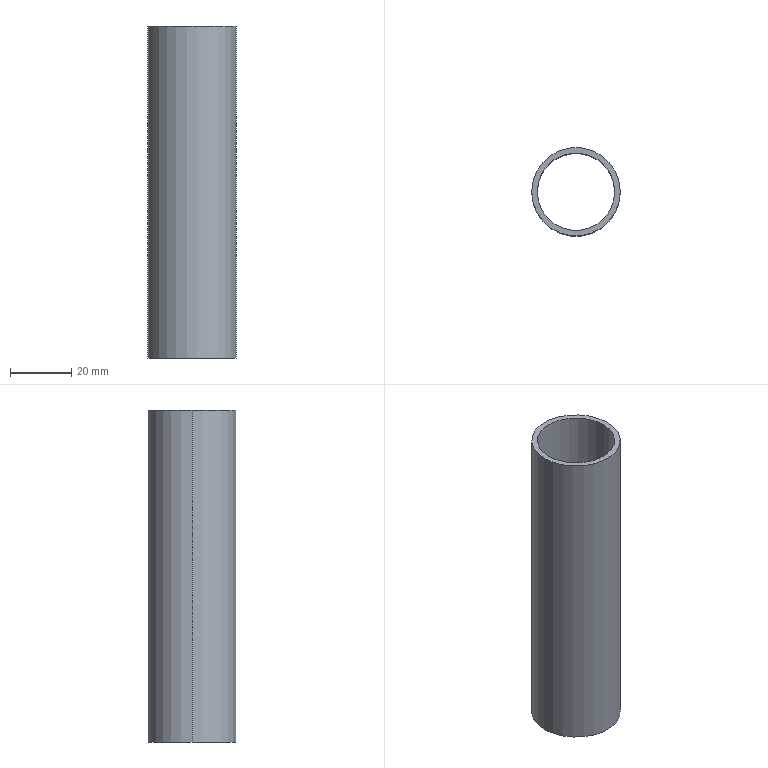Part | SolidWorks | features Extrusion 1 | 1 solid | 6 faces | box 28.8 x 28.8 x 108 mm | volume 16490 mm3 | cylinder 4 | plane 2 | commonest cylinder face diameters 25.2 x2 28.8 x2
STEP:
#1=CARTESIAN_POINT('',(-12.6,0.,108.));
#2=VERTEX_POINT('',#1);
#3=CARTESIAN_POINT('',(12.6,0.,108.));
#4=VERTEX_POINT('',#3);
#5=CARTESIAN_POINT('',(0.,0.,108.));
#6=DIRECTION('',(0.,0.,1.));
#7=DIRECTION('',(1.,0.,0.));
#8=AXIS2_PLACEMENT_3D('',#5,#6,#7);
#9=CIRCLE('',#8,12.6);
#10=EDGE_CURVE('',#2,#4,#9,.T.);
#11=ORIENTED_EDGE('',*,*,#10,.T.);
#12=CARTESIAN_POINT('',(12.6,0.,0.));
#13=VERTEX_POINT('',#12);
#14=CARTESIAN_POINT('',(12.6,0.,108.));
#15=DIRECTION('',(0.,0.,-1.));
#16=VECTOR('',#15,1000.);
#17=LINE('',#14,#16);
#18=EDGE_CURVE('',#4,#13,#17,.T.);
#19=ORIENTED_EDGE('',*,*,#18,.T.);
#20=CARTESIAN_POINT('',(-12.6,0.,0.));
#21=VERTEX_POINT('',#20);
#22=CARTESIAN_POINT('',(0.,0.,0.));
#23=DIRECTION('',(0.,0.,1.));
#24=DIRECTION('',(1.,0.,0.));
#25=AXIS2_PLACEMENT_3D('',#22,#23,#24);
#26=CIRCLE('',#25,12.6);
#27=EDGE_CURVE('',#21,#13,#26,.T.);
#28=ORIENTED_EDGE('',*,*,#27,.F.);
#29=CARTESIAN_POINT('',(-12.6,0.,108.));
#30=DIRECTION('',(0.,0.,-1.));
#31=VECTOR('',#30,1000.);
#32=LINE('',#29,#31);
#33=EDGE_CURVE('',#2,#21,#32,.T.);
#34=ORIENTED_EDGE('',*,*,#33,.F.);
#35=EDGE_LOOP('',(#11,#19,#28,#34));
#36=FACE_OUTER_BOUND('',#35,.T.);
#37=CARTESIAN_POINT('',(0.,0.,108.));
#38=DIRECTION('',(0.,0.,-1.));
#39=DIRECTION('',(-1.,0.,0.));
#40=AXIS2_PLACEMENT_3D('',#37,#38,#39);
#41=CYLINDRICAL_SURFACE('',#40,12.6);
#42=ADVANCED_FACE('',(#36),#41,.F.);
#43=CARTESIAN_POINT('',(14.4,0.,108.));
#44=VERTEX_POINT('',#43);
#45=CARTESIAN_POINT('',(-14.4,0.,108.));
#46=VERTEX_POINT('',#45);
#47=CARTESIAN_POINT('',(0.,0.,108.));
#48=DIRECTION('',(0.,0.,1.));
#49=DIRECTION('',(1.,0.,0.));
#50=AXIS2_PLACEMENT_3D('',#47,#48,#49);
#51=CIRCLE('',#50,14.4);
#52=EDGE_CURVE('',#44,#46,#51,.T.);
#53=ORIENTED_EDGE('',*,*,#52,.F.);
#54=CARTESIAN_POINT('',(14.4,0.,0.));
#55=VERTEX_POINT('',#54);
#56=CARTESIAN_POINT('',(14.4,0.,108.));
#57=DIRECTION('',(0.,0.,-1.));
#58=VECTOR('',#57,1000.);
#59=LINE('',#56,#58);
#60=EDGE_CURVE('',#44,#55,#59,.T.);
#61=ORIENTED_EDGE('',*,*,#60,.T.);
#62=CARTESIAN_POINT('',(-14.4,0.,0.));
#63=VERTEX_POINT('',#62);
#64=CARTESIAN_POINT('',(0.,0.,0.));
#65=DIRECTION('',(0.,0.,1.));
#66=DIRECTION('',(1.,0.,0.));
#67=AXIS2_PLACEMENT_3D('',#64,#65,#66);
#68=CIRCLE('',#67,14.4);
#69=EDGE_CURVE('',#55,#63,#68,.T.);
#70=ORIENTED_EDGE('',*,*,#69,.T.);
#71=CARTESIAN_POINT('',(-14.4,0.,108.));
#72=DIRECTION('',(0.,0.,-1.));
#73=VECTOR('',#72,1000.);
#74=LINE('',#71,#73);
#75=EDGE_CURVE('',#46,#63,#74,.T.);
#76=ORIENTED_EDGE('',*,*,#75,.F.);
#77=EDGE_LOOP('',(#53,#61,#70,#76));
#78=FACE_OUTER_BOUND('',#77,.T.);
#79=CARTESIAN_POINT('',(0.,0.,108.));
#80=DIRECTION('',(0.,0.,-1.));
#81=DIRECTION('',(-1.,0.,0.));
#82=AXIS2_PLACEMENT_3D('',#79,#80,#81);
#83=CYLINDRICAL_SURFACE('',#82,14.4);
#84=ADVANCED_FACE('',(#78),#83,.T.);
#85=CARTESIAN_POINT('',(0.,0.,108.));
#86=DIRECTION('',(0.,0.,1.));
#87=DIRECTION('',(1.,0.,0.));
#88=AXIS2_PLACEMENT_3D('',#85,#86,#87);
#89=CIRCLE('',#88,14.4);
#90=EDGE_CURVE('',#46,#44,#89,.T.);
#91=ORIENTED_EDGE('',*,*,#90,.T.);
#92=ORIENTED_EDGE('',*,*,#52,.T.);
#93=EDGE_LOOP('',(#91,#92));
#94=FACE_OUTER_BOUND('',#93,.T.);
#95=ORIENTED_EDGE('',*,*,#10,.F.);
#96=CARTESIAN_POINT('',(0.,0.,108.));
#97=DIRECTION('',(0.,0.,1.));
#98=DIRECTION('',(1.,0.,0.));
#99=AXIS2_PLACEMENT_3D('',#96,#97,#98);
#100=CIRCLE('',#99,12.6);
#101=EDGE_CURVE('',#4,#2,#100,.T.);
#102=ORIENTED_EDGE('',*,*,#101,.F.);
#103=EDGE_LOOP('',(#95,#102));
#104=FACE_BOUND('',#103,.T.);
#105=CARTESIAN_POINT('',(0.,0.,108.));
#106=DIRECTION('',(0.,0.,1.));
#107=DIRECTION('',(1.,0.,0.));
#108=AXIS2_PLACEMENT_3D('',#105,#106,#107);
#109=PLANE('',#108);
#110=ADVANCED_FACE('',(#94,#104),#109,.T.);
#111=CARTESIAN_POINT('',(0.,0.,0.));
#112=DIRECTION('',(0.,0.,1.));
#113=DIRECTION('',(1.,0.,0.));
#114=AXIS2_PLACEMENT_3D('',#111,#112,#113);
#115=CIRCLE('',#114,14.4);
#116=EDGE_CURVE('',#63,#55,#115,.T.);
#117=ORIENTED_EDGE('',*,*,#116,.F.);
#118=ORIENTED_EDGE('',*,*,#69,.F.);
#119=EDGE_LOOP('',(#117,#118));
#120=FACE_OUTER_BOUND('',#119,.T.);
#121=ORIENTED_EDGE('',*,*,#27,.T.);
#122=CARTESIAN_POINT('',(0.,0.,0.));
#123=DIRECTION('',(0.,0.,1.));
#124=DIRECTION('',(1.,0.,0.));
#125=AXIS2_PLACEMENT_3D('',#122,#123,#124);
#126=CIRCLE('',#125,12.6);
#127=EDGE_CURVE('',#13,#21,#126,.T.);
#128=ORIENTED_EDGE('',*,*,#127,.T.);
#129=EDGE_LOOP('',(#121,#128));
#130=FACE_BOUND('',#129,.T.);
#131=CARTESIAN_POINT('',(0.,0.,0.));
#132=DIRECTION('',(0.,0.,1.));
#133=DIRECTION('',(1.,0.,0.));
#134=AXIS2_PLACEMENT_3D('',#131,#132,#133);
#135=PLANE('',#134);
#136=ADVANCED_FACE('',(#120,#130),#135,.F.);
#137=ORIENTED_EDGE('',*,*,#60,.F.);
#138=ORIENTED_EDGE('',*,*,#90,.F.);
#139=ORIENTED_EDGE('',*,*,#75,.T.);
#140=ORIENTED_EDGE('',*,*,#116,.T.);
#141=EDGE_LOOP('',(#137,#138,#139,#140));
#142=FACE_OUTER_BOUND('',#141,.T.);
#143=CARTESIAN_POINT('',(0.,0.,108.));
#144=DIRECTION('',(0.,0.,-1.));
#145=DIRECTION('',(-1.,0.,0.));
#146=AXIS2_PLACEMENT_3D('',#143,#144,#145);
#147=CYLINDRICAL_SURFACE('',#146,14.4);
#148=ADVANCED_FACE('',(#142),#147,.T.);
#149=ORIENTED_EDGE('',*,*,#18,.F.);
#150=ORIENTED_EDGE('',*,*,#101,.T.);
#151=ORIENTED_EDGE('',*,*,#33,.T.);
#152=ORIENTED_EDGE('',*,*,#127,.F.);
#153=EDGE_LOOP('',(#149,#150,#151,#152));
#154=FACE_OUTER_BOUND('',#153,.T.);
#155=CARTESIAN_POINT('',(0.,0.,108.));
#156=DIRECTION('',(0.,0.,-1.));
#157=DIRECTION('',(-1.,0.,0.));
#158=AXIS2_PLACEMENT_3D('',#155,#156,#157);
#159=CYLINDRICAL_SURFACE('',#158,12.6);
#160=ADVANCED_FACE('',(#154),#159,.F.);
#161=CLOSED_SHELL('',(#42,#84,#110,#136,#148,#160));
#162=MANIFOLD_SOLID_BREP('',#161);
#163=CARTESIAN_POINT('',(0.,0.,0.));
#164=DIRECTION('',(0.,0.,1.));
#165=DIRECTION('',(1.,0.,0.));
#166=AXIS2_PLACEMENT_3D('',#163,#164,#165);
#167=(LENGTH_UNIT()NAMED_UNIT(*)SI_UNIT(.MILLI.,.METRE.));
#168=UNCERTAINTY_MEASURE_WITH_UNIT(LENGTH_MEASURE(0.00001),#167,'','');
#169=(NAMED_UNIT(*)PLANE_ANGLE_UNIT()SI_UNIT($,.RADIAN.));
#170=(NAMED_UNIT(*)SI_UNIT($,.STERADIAN.)SOLID_ANGLE_UNIT());
#171=(GEOMETRIC_REPRESENTATION_CONTEXT(3)GLOBAL_UNCERTAINTY_ASSIGNED_CONTEXT((#168))GLOBAL_UNIT_ASSIGNED_CONTEXT((#167,#169,#170))REPRESENTATION_CONTEXT('',''));
#172=ADVANCED_BREP_SHAPE_REPRESENTATION('',(#162,#166),#171);